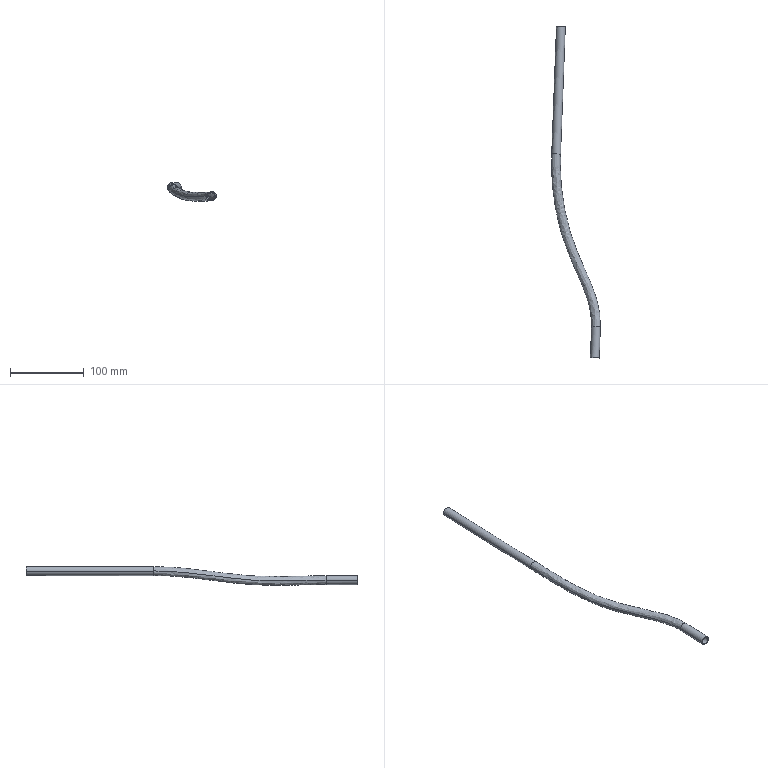Part | SolidWorks | features 3DProfileFeature 2, Sweep 1 | 1 solid | 14 faces | box 66.294 x 450.059 x 25.234 mm | volume 15866 mm3 | cylinder 8 | spline 4 | plane 2 | commonest cylinder face diameters 10 x4 12 x4